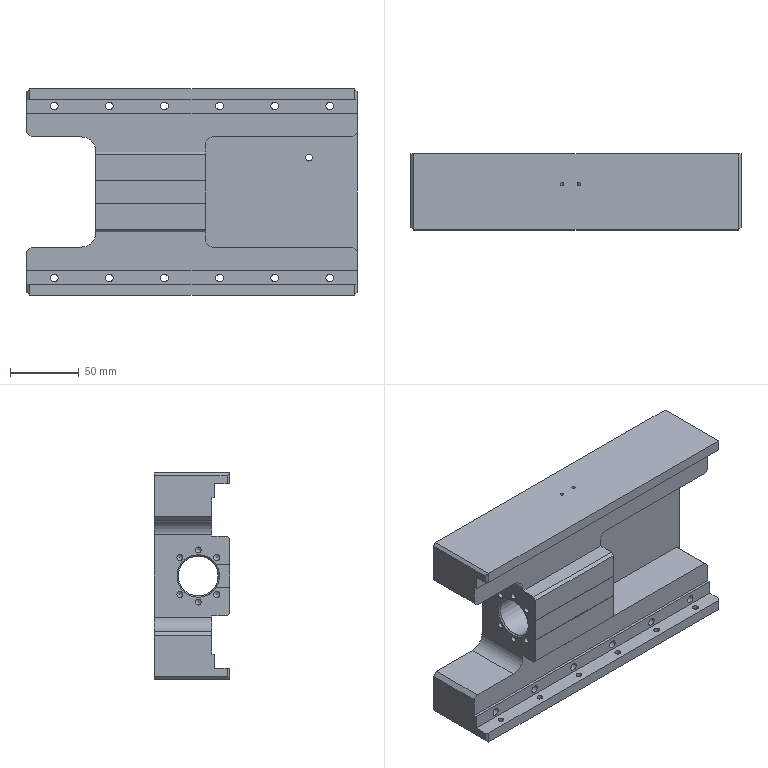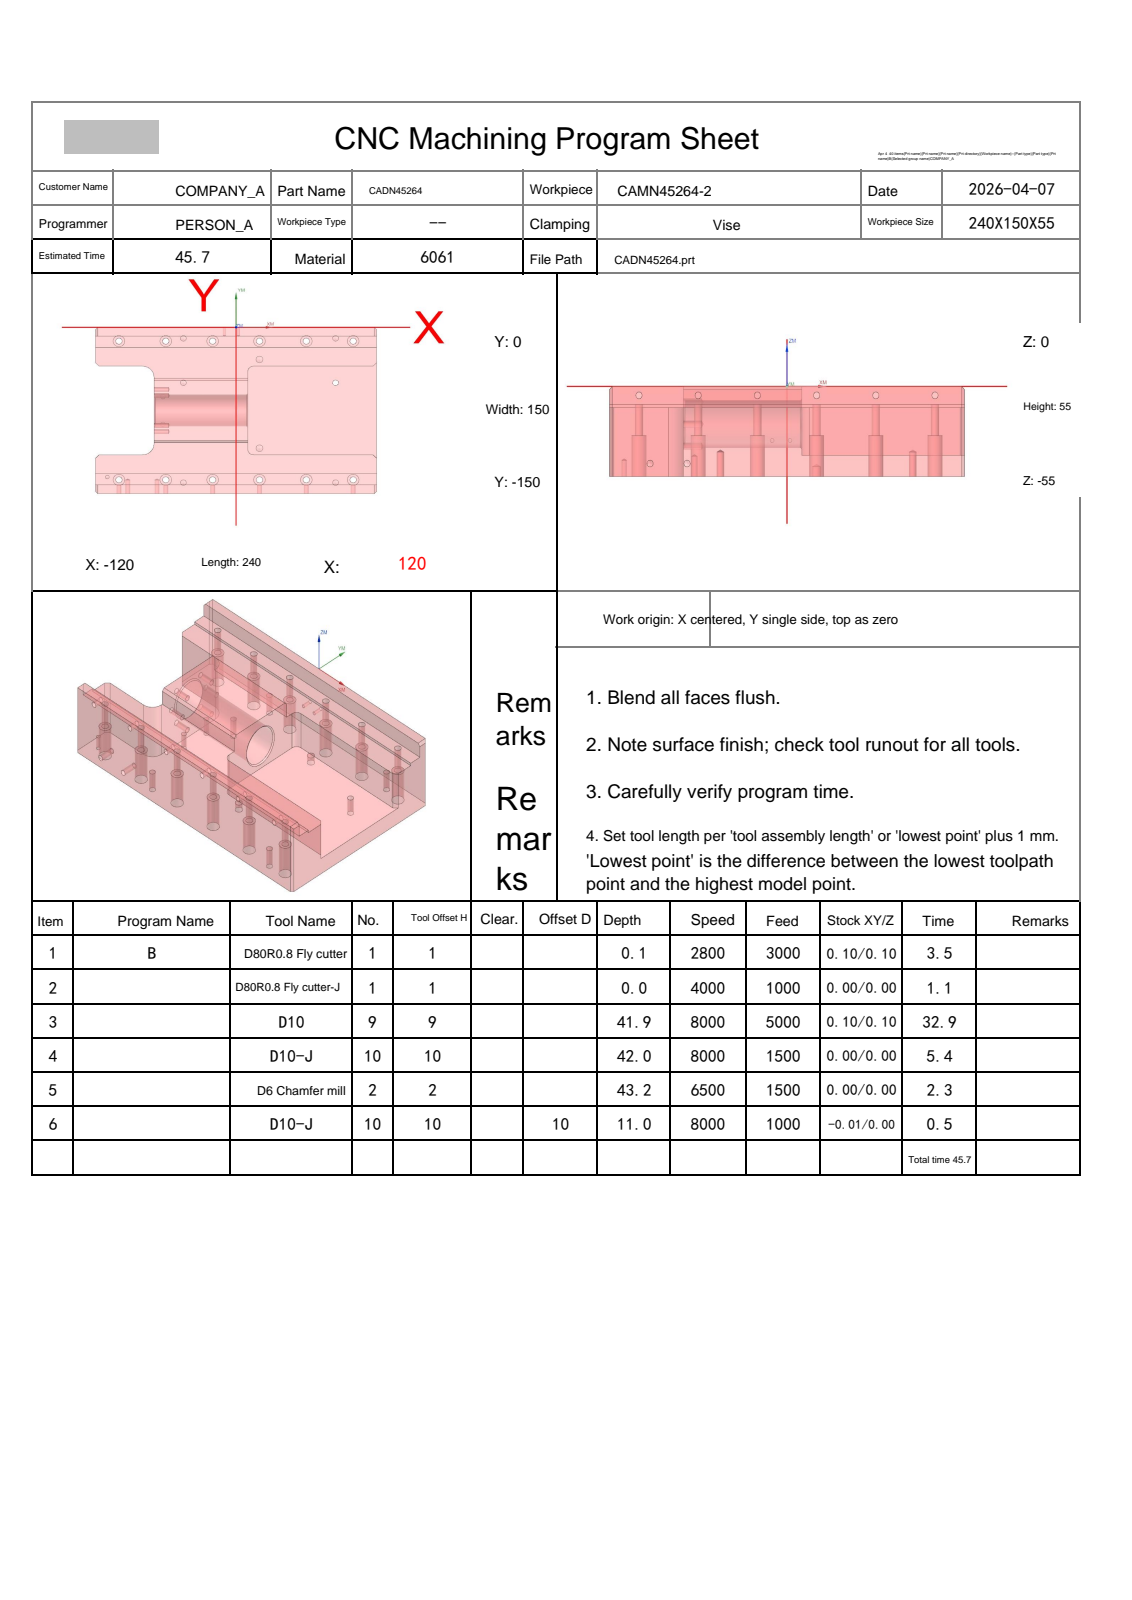NC program | NX | posted by the shop | part box 240 x 55 x 150 mm
Lines 1 to 208 of 15848:
%
O0001
(Machine time: 46.59 MIN)
(===Total Tool:4===)
(T1=D80R0.8 Fly cutter D=80.  R=0.8  D-  H01 Z=0.    )
(T9=D10     D=10.  R=0.   D-  H09 Z=-41.9 )
(T10=D10-J  D=10.  R=0.   D10 H10 Z=-42.  )
(T2=D6 Chamfer mill   D=6.   R=0.   D-  H02 Z=-43.2 )
G80 G90 G17 G49 G40
G91 G28 Z0
M01
N1 T01 M06
(D80R0.8 Fly cutter  D=80. R=0.8 H=01 ce=0.10 di=0.10)
G00 G90 G54 X172.097 Y-126.097 M03 S2800
G43 H01 Z50.
M08
Z6.011
G01 Z4.011 F3000.
X160.097
X-152.1
G02 X-160.097 Y-118.101 I.003 J8.
G01 Y-104.704
G02 X-157.755 Y-99.049 I8. J-.001
G01 X-139.726 Y-81.021
G02 X-134.076 Y-78.68 I5.654 J-5.659
G01 X152.897
G03 X160.097 Y-71.48 I0.0 J7.2
G01 Y-39.263
G03 X152.097 Y-31.263 I-8. J0.0
G01 X-160.097
X-172.097
Z6.011
G00 X172.097 Y-126.097
Z5.522
G01 Z3.522
X160.097
X-152.1
G02 X-160.097 Y-118.101 I.003 J8.
G01 Y-104.704
G02 X-157.755 Y-99.049 I8. J-.001
G01 X-139.726 Y-81.021
G02 X-134.076 Y-78.68 I5.654 J-5.659
G01 X152.897
G03 X160.097 Y-71.48 I0.0 J7.2
G01 Y-39.263
G03 X152.097 Y-31.263 I-8. J0.0
G01 X-160.097
X-172.097
Z5.522
G00 X172.097 Y-126.097
Z5.033
G01 Z3.033
X160.097
X-152.1
G02 X-160.097 Y-118.101 I.003 J8.
G01 Y-104.704
G02 X-157.755 Y-99.049 I8. J-.001
G01 X-139.726 Y-81.021
G02 X-134.076 Y-78.68 I5.654 J-5.659
G01 X152.897
G03 X160.097 Y-71.48 I0.0 J7.2
G01 Y-39.263
G03 X152.097 Y-31.263 I-8. J0.0
G01 X-160.097
X-172.097
Z5.033
G00 X172.097 Y-126.097
Z4.544
G01 Z2.544
X160.097
X-152.1
G02 X-160.097 Y-118.101 I.003 J8.
G01 Y-104.704
G02 X-157.755 Y-99.049 I8. J-.001
G01 X-139.726 Y-81.021
G02 X-134.076 Y-78.68 I5.654 J-5.659
G01 X152.897
G03 X160.097 Y-71.48 I0.0 J7.2
G01 Y-39.263
G03 X152.097 Y-31.263 I-8. J0.0
G01 X-160.097
X-172.097
Z4.544
G00 Z50.
X172.097 Y-126.097
Z4.056
G01 Z2.056
X160.097
X-152.1
G02 X-160.097 Y-118.101 I.003 J8.
G01 Y-104.704
G02 X-157.755 Y-99.049 I8. J-.001
G01 X-139.726 Y-81.021
G02 X-134.076 Y-78.68 I5.654 J-5.659
G01 X152.897
G03 X160.097 Y-71.48 I0.0 J7.2
G01 Y-39.263
G03 X152.097 Y-31.263 I-8. J0.0
G01 X-160.097
X-172.097
Z4.056
G00 Z50.
X172.097 Y-126.097
Z3.567
G01 Z1.567
X160.097
X-152.1
G02 X-160.097 Y-118.101 I.003 J8.
G01 Y-104.704
G02 X-157.755 Y-99.049 I8. J-.001
G01 X-139.726 Y-81.021
G02 X-134.076 Y-78.68 I5.654 J-5.659
G01 X152.897
G03 X160.097 Y-71.48 I0.0 J7.2
G01 Y-39.263
G03 X152.097 Y-31.263 I-8. J0.0
G01 X-160.097
X-172.097
Z3.567
G00 Z50.
X172.097 Y-126.097
Z3.078
G01 Z1.078
X160.097
X-152.1
G02 X-160.097 Y-118.101 I.003 J8.
G01 Y-104.704
G02 X-157.755 Y-99.049 I8. J-.001
G01 X-139.726 Y-81.021
G02 X-134.076 Y-78.68 I5.654 J-5.659
G01 X152.897
G03 X160.097 Y-71.48 I0.0 J7.2
G01 Y-39.263
G03 X152.097 Y-31.263 I-8. J0.0
G01 X-160.097
X-172.097
Z3.078
G00 Z50.
X172.097 Y-126.097
Z2.589
G01 Z.589
X160.097
X-152.1
G02 X-160.097 Y-118.101 I.003 J8.
G01 Y-104.704
G02 X-157.755 Y-99.049 I8. J-.001
G01 X-139.726 Y-81.021
G02 X-134.076 Y-78.68 I5.654 J-5.659
G01 X152.897
G03 X160.097 Y-71.48 I0.0 J7.2
G01 Y-39.263
G03 X152.097 Y-31.263 I-8. J0.0
G01 X-160.097
X-172.097
Z2.589
G00 Z50.
X172.097 Y-126.097
Z2.1
G01 Z.1
X160.097
X-152.1
G02 X-160.097 Y-118.101 I.003 J8.
G01 Y-104.704
G02 X-157.755 Y-99.049 I8. J-.001
G01 X-139.726 Y-81.021
G02 X-134.076 Y-78.68 I5.654 J-5.659
G01 X152.897
G03 X160.097 Y-71.48 I0.0 J7.2
G01 Y-39.263
G03 X152.097 Y-31.263 I-8. J0.0
G01 X-160.097
X-172.097
Z2.1
G00 Z50.
G91 G28 Z0.0
M05
M09
G91 G28 Z0.0
M01
N2 T01 M06
(D80R0.8 Fly cutter-J  D=80. R=0.8 H=01 ce=0.00 di=0.00)
G00 G90 G54 X171.999 Y-125.999 M03 S4000
G43 H01 Z50.
M08
Z2.
G01 Z0.0 F1000.
X159.999
X-152.002
G02 X-159.999 Y-118.003 I.003 J8.
G01 Y-104.744
G02 X-157.657 Y-99.09 I8. J-.001
G01 X-139.588 Y-81.021
G02 X-133.937 Y-78.68 I5.654 J-5.659
G01 X152.799
G03 X159.999 Y-71.48 I0.0 J7.2
G01 Y-39.361
G03 X151.999 Y-31.361 I-8. J0.0
G01 X-159.999
X-171.999
Z2.
G00 Z50.
G91 G28 Z0.0
M05
M09
G91 G28 Z0.0
M01